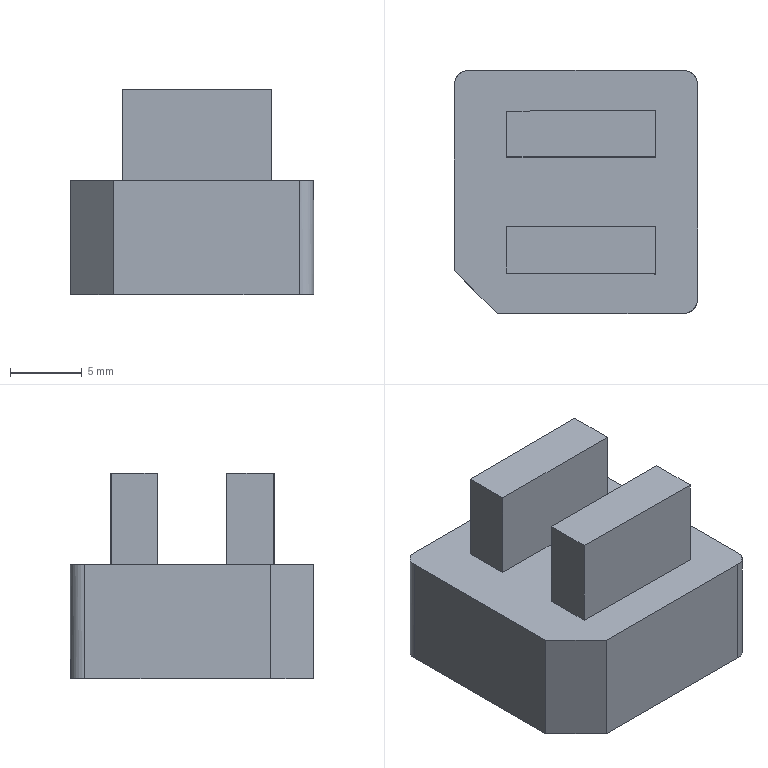NC program | PowerMill | posted with a generic post | part box 17 x 17 x 14.396 mm
Lines 2717 to 3695 of 69084:
N2814 M6
N2815 S18000 M03
N2816 G00 G90 X0.0 Y0.0
N2817 G43 Z9.7958 H15
N2818
N2819 G05 P10000 R4
N2820 X1.635 Y-8.1486
N2821 Z0.8391
N2822 G01 Z-0.3609 F3000.0
N2823 X1.6437 Y-8.1314 F5000.0
N2824 G03 X1.5675 Y-7.8985 I-0.1545 J0.0783
N2825 G01 X0.2111 Y-7.2114
N2826 X-4.8545 Y-7.1849
N2827 X-5.2767 Y-7.1304
N2828 X-5.6576 Y-6.9652
N2829 X-6.1064 Y-6.5431
N2830 X-6.3115 Y-6.1209
N2831 X-6.3761 Y-5.6988
N2832 X-6.3724 Y-2.3217
N2833 X-6.2796 Y-1.8996
N2834 X-6.1209 Y-1.592
N2835 X-6.0357 Y-1.4775
N2836 X-5.6988 Y-1.1748
N2837 X-5.4786 Y-1.0553
N2838 X-5.2767 Y-0.9836
N2839 X-4.8545 Y-0.9292
N2840 X5.2767
N2841 X5.6988 Y-0.9368
N2842 X6.1209 Y-1.0428
N2843 X6.5431 Y-1.3066
N2844 X6.7076 Y-1.4775
N2845 X6.9516 Y-1.8996
N2846 X7.0443 Y-2.3217
N2847 X7.0482 Y-5.6988
N2848 X6.9988 Y-6.1209
N2849 X6.8147 Y-6.5431
N2850 X6.5431 Y-6.8619
N2851 X6.4127 Y-6.9652
N2852 X6.1209 Y-7.1257
N2853 X5.6988 Y-7.2318
N2854 X5.2767 Y-7.238
N2855 X0.2111 Y-7.2114
N2856 G00 Z5.7953
N2857 G01 X-1.9723 Y-0.8992 F10000.0
N2858 G00 Z-0.1109
N2859 G01 X-2.2978 Z-0.1166 F3000.0
N2860 X-4.8545 Z-0.1612
N2861 X-4.8584 Y-0.8994
N2862 X-5.147 Y-0.9366 Z-0.1663
N2863 X-5.1478 Y-0.9292 Z-0.1665
N2864 X-5.093 Y-0.3731 Z-0.1762
N2865 X-4.9308 Y0.1615 Z-0.186
N2866 X-4.6675 Y0.6542 Z-0.1957
N2867 X-4.4661 Y0.8996 Z-0.2012
N2868 X-0.1294 Y0.8995 Z-0.2769
N2869 X0.0719 Y0.6542 Z-0.2825
N2870 X0.3353 Y0.1615 Z-0.2922
N2871 X0.4975 Y-0.3731 Z-0.302
N2872 X0.5493 Y-0.8992 Z-0.3112
N2873 X-2.2978 Z-0.3609
N2874 Y-0.9292
N2875 X-4.8756 Y0.9331 F5000.0
N2876 X-5.2767 Y0.9986
N2877 X-5.4279 Y1.0553
N2878 X-5.6988 Y1.2093
N2879 X-5.9855 Y1.4775
N2880 X-6.1209 Y1.6719
N2881 X-6.2295 Y1.8996
N2882 X-6.3223 Y2.3217
N2883 X-6.3249 Y5.6988
N2884 X-6.2454 Y6.1209
N2885 X-6.1209 Y6.3928
N2886 X-6.0204 Y6.5431
N2887 X-5.6988 Y6.8554
N2888 X-5.5201 Y6.9652
N2889 X-5.2767 Y7.0661
N2890 X-4.8545 Y7.135
N2891 X5.2767 Y7.1883
N2892 X5.6988 Y7.1821
N2893 X6.1209 Y7.0759
N2894 X6.3374 Y6.9652
N2895 X6.5431 Y6.8122
N2896 X6.7817 Y6.5431
N2897 X6.9652 Y6.1816
N2898 X7.0481 Y5.6988
N2899 X7.0442 Y2.3217
N2900 X6.9652 Y1.9374
N2901 X6.7074 Y1.4775
N2902 X6.5431 Y1.3068
N2903 X6.1499 Y1.0553
N2904 X5.6988 Y0.9369
N2905 X5.2767 Y0.9294
N2906 X-4.8545 Y0.9296
N2907 X-4.8756 Y0.9331
N2908 X-6.6768 Y-0.018 Z-0.5078
N2909 X-6.5047 Y-0.1041
N2910 X-4.8545 Y-0.9292
N2911 X5.2767
N2912 X5.6988 Y-0.9368
N2913 X6.1209 Y-1.0428
N2914 X6.5431 Y-1.3066
N2915 X6.7076 Y-1.4775
N2916 X6.9516 Y-1.8996
N2917 X7.0443 Y-2.3217
N2918 X7.0482 Y-5.6988
N2919 X6.9988 Y-6.1209
N2920 X6.8147 Y-6.5431
N2921 X6.5431 Y-6.8619
N2922 X6.4127 Y-6.9652
N2923 X6.1209 Y-7.1257
N2924 X5.6988 Y-7.2318
N2925 X5.2767 Y-7.238
N2926 X-4.8545 Y-7.1849
N2927 X-5.2767 Y-7.1304
N2928 X-5.6576 Y-6.9652
N2929 X-6.1064 Y-6.5431
N2930 X-6.3115 Y-6.1209
N2931 X-6.3761 Y-5.6988
N2932 X-6.3724 Y-2.3217
N2933 X-6.2796 Y-1.8996
N2934 X-6.1209 Y-1.592
N2935 X-6.0357 Y-1.4775
N2936 X-5.6988 Y-1.1748
N2937 X-5.4786 Y-1.0553
N2938 X-5.2767 Y-0.9836
N2939 X-4.8545 Y-0.9292
N2940 X-2.0017 Y-0.8992 Z-0.2578
N2941 X-2.3239 Z-0.2634 F3000.0
N2942 X-4.8545 Z-0.3075
N2943 X-4.8584 Y-0.8994 Z-0.3076
N2944 X-5.1729 Y-0.9399 Z-0.3131
N2945 X-5.1739 Y-0.9292 Z-0.3133
N2946 X-5.1192 Y-0.3731 Z-0.3231
N2947 X-4.957 Y0.1615 Z-0.3328
N2948 X-4.6936 Y0.6542 Z-0.3426
N2949 X-4.4922 Y0.8996 Z-0.3481
N2950 X-0.1556 Y0.8995 Z-0.4238
N2951 X0.0458 Y0.6542 Z-0.4293
N2952 X0.3091 Y0.1615 Z-0.4391
N2953 X0.4713 Y-0.3731 Z-0.4488
N2954 X0.5231 Y-0.8992 Z-0.4581
N2955 X-2.3239 Z-0.5078
N2956 Y-0.9292
N2957 X-4.9094 Y0.9386 F5000.0
N2958 X-5.2767 Y0.9986
N2959 X-5.4279 Y1.0553
N2960 X-5.6988 Y1.2093
N2961 X-5.9855 Y1.4775
N2962 X-6.1209 Y1.6719
N2963 X-6.2295 Y1.8996
N2964 X-6.3223 Y2.3217
N2965 X-6.3249 Y5.6988
N2966 X-6.2454 Y6.1209
N2967 X-6.1209 Y6.3928
N2968 X-6.0204 Y6.5431
N2969 X-5.6988 Y6.8554
N2970 X-5.5201 Y6.9652
N2971 X-5.2767 Y7.0661
N2972 X-4.8545 Y7.135
N2973 X5.2767 Y7.1883
N2974 X5.6988 Y7.1821
N2975 X6.1209 Y7.0759
N2976 X6.3374 Y6.9652
N2977 X6.5431 Y6.8122
N2978 X6.7817 Y6.5431
N2979 X6.9652 Y6.1816
N2980 X7.0481 Y5.6988
N2981 X7.0442 Y2.3217
N2982 X6.9652 Y1.9374
N2983 X6.7074 Y1.4775
N2984 X6.5431 Y1.3068
N2985 X6.1499 Y1.0553
N2986 X5.6988 Y0.9369
N2987 X5.2767 Y0.9294
N2988 X-4.8545 Y0.9296
N2989 X-4.9094 Y0.9386
N2990 X-6.6768 Y-0.018 Z-0.6546
N2991 X-6.5047 Y-0.1041
N2992 X-4.8545 Y-0.9291
N2993 X5.2767
N2994 X5.6988 Y-0.9368
N2995 X6.1209 Y-1.0428
N2996 X6.5431 Y-1.3066
N2997 X6.7076 Y-1.4775
N2998 X6.9516 Y-1.8996
N2999 X7.0443 Y-2.3217
N3000 X7.0482 Y-5.6988
N3001 X6.9988 Y-6.1209
N3002 X6.8147 Y-6.5431
N3003 X6.5431 Y-6.8619
N3004 X6.4127 Y-6.9652
N3005 X6.1209 Y-7.1257
N3006 X5.6988 Y-7.2318
N3007 X5.2767 Y-7.238
N3008 X-4.8545 Y-7.1849
N3009 X-5.2767 Y-7.1304
N3010 X-5.6576 Y-6.9652
N3011 X-6.1064 Y-6.5431
N3012 X-6.3115 Y-6.1209
N3013 X-6.3761 Y-5.6988
N3014 X-6.3724 Y-2.3217
N3015 X-6.2796 Y-1.8996
N3016 X-6.1209 Y-1.592
N3017 X-6.0357 Y-1.4775
N3018 X-5.6988 Y-1.1748
N3019 X-5.4786 Y-1.0553
N3020 X-5.2767 Y-0.9836
N3021 X-4.8545 Y-0.9291
N3022 X-2.0017 Y-0.8991 Z-0.4046
N3023 X-2.3239 Z-0.4103 F3000.0
N3024 X-4.8545 Z-0.4544
N3025 X-4.8584 Y-0.8994 Z-0.4545
N3026 X-5.1729 Y-0.9399 Z-0.46
N3027 X-5.1739 Y-0.9291 Z-0.4602
N3028 X-5.1192 Y-0.3731 Z-0.47
N3029 X-4.957 Y0.1615 Z-0.4797
N3030 X-4.6936 Y0.6542 Z-0.4895
N3031 X-4.4922 Y0.8996 Z-0.495
N3032 X-0.1556 Y0.8995 Z-0.5707
N3033 X0.0458 Y0.6542 Z-0.5762
N3034 X0.3091 Y0.1615 Z-0.586
N3035 X0.4713 Y-0.3731 Z-0.5957
N3036 X0.5231 Y-0.8991 Z-0.605
N3037 X-2.3239 Z-0.6546
N3038 Y-0.9291
N3039 X-4.9094 Y0.9386 F5000.0
N3040 X-5.2767 Y0.9986
N3041 X-5.4279 Y1.0553
N3042 X-5.6988 Y1.2092
N3043 X-5.9855 Y1.4775
N3044 X-6.1209 Y1.6719
N3045 X-6.2295 Y1.8996
N3046 X-6.3223 Y2.3217
N3047 X-6.3249 Y5.6988
N3048 X-6.2454 Y6.1209
N3049 X-6.1209 Y6.3928
N3050 X-6.0204 Y6.5431
N3051 X-5.6988 Y6.8554
N3052 X-5.5201 Y6.9652
N3053 X-5.2767 Y7.0661
N3054 X-4.8545 Y7.1351
N3055 X5.2767 Y7.1883
N3056 X5.6988 Y7.1821
N3057 X6.1209 Y7.0759
N3058 X6.3375 Y6.9652
N3059 X6.5431 Y6.8122
N3060 X6.7817 Y6.5431
N3061 X6.9652 Y6.1816
N3062 X7.0481 Y5.6988
N3063 X7.0442 Y2.3217
N3064 X6.9652 Y1.9374
N3065 X6.7074 Y1.4775
N3066 X6.5431 Y1.3068
N3067 X6.1499 Y1.0553
N3068 X5.6988 Y0.9369
N3069 X5.2767 Y0.9294
N3070 X-4.8545 Y0.9296
N3071 X-4.9094 Y0.9386
N3072 X-6.6768 Y-0.018 Z-0.8015
N3073 X-6.5047 Y-0.1041
N3074 X-4.8545 Y-0.9291
N3075 X5.2767
N3076 X5.6988 Y-0.9367
N3077 X6.1209 Y-1.0428
N3078 X6.5431 Y-1.3066
N3079 X6.7076 Y-1.4775
N3080 X6.9516 Y-1.8996
N3081 X7.0443 Y-2.3217
N3082 X7.0482 Y-5.6988
N3083 X6.9988 Y-6.1209
N3084 X6.8147 Y-6.5431
N3085 X6.5431 Y-6.8619
N3086 X6.4127 Y-6.9652
N3087 X6.1209 Y-7.1257
N3088 X5.6988 Y-7.2318
N3089 X5.2767 Y-7.238
N3090 X-4.8545 Y-7.1849
N3091 X-5.2767 Y-7.1304
N3092 X-5.6576 Y-6.9652
N3093 X-6.1064 Y-6.5431
N3094 X-6.3115 Y-6.1209
N3095 X-6.3761 Y-5.6988
N3096 X-6.3724 Y-2.3217
N3097 X-6.2797 Y-1.8996
N3098 X-6.1209 Y-1.592
N3099 X-6.0357 Y-1.4775
N3100 X-5.6988 Y-1.1748
N3101 X-5.4786 Y-1.0553
N3102 X-5.2767 Y-0.9836
N3103 X-4.8545 Y-0.9291
N3104 X-2.0017 Y-0.8991 Z-0.5515
N3105 X-2.3239 Z-0.5572 F3000.0
N3106 X-4.8545 Z-0.6013
N3107 X-4.8584 Y-0.8994 Z-0.6014
N3108 X-5.1729 Y-0.9399 Z-0.6069
N3109 X-5.1739 Y-0.9291 Z-0.6071
N3110 X-5.1192 Y-0.3731 Z-0.6169
N3111 X-4.957 Y0.1615 Z-0.6266
N3112 X-4.6936 Y0.6542 Z-0.6364
N3113 X-4.4922 Y0.8996 Z-0.6419
N3114 X-0.1556 Y0.8995 Z-0.7176
N3115 X0.0457 Y0.6542 Z-0.7231
N3116 X0.3091 Y0.1615 Z-0.7329
N3117 X0.4713 Y-0.3731 Z-0.7426
N3118 X0.5231 Y-0.8991 Z-0.7518
N3119 X-2.3239 Z-0.8015
N3120 Y-0.9291
N3121 X-4.9094 Y0.9386 F5000.0
N3122 X-5.2767 Y0.9986
N3123 X-5.4279 Y1.0553
N3124 X-5.6988 Y1.2092
N3125 X-5.9855 Y1.4775
N3126 X-6.1209 Y1.6719
N3127 X-6.2295 Y1.8996
N3128 X-6.3223 Y2.3217
N3129 X-6.3249 Y5.6988
N3130 X-6.2454 Y6.1209
N3131 X-6.1209 Y6.3928
N3132 X-6.0204 Y6.5431
N3133 X-5.6988 Y6.8554
N3134 X-5.5201 Y6.9652
N3135 X-5.2767 Y7.0661
N3136 X-4.8545 Y7.1351
N3137 X5.2767 Y7.1883
N3138 X5.6988 Y7.1821
N3139 X6.1209 Y7.0759
N3140 X6.3375 Y6.9652
N3141 X6.5431 Y6.8122
N3142 X6.7817 Y6.5431
N3143 X6.9652 Y6.1816
N3144 X7.0481 Y5.6988
N3145 X7.0442 Y2.3217
N3146 X6.9652 Y1.9374
N3147 X6.7074 Y1.4775
N3148 X6.5431 Y1.3068
N3149 X6.1499 Y1.0553
N3150 X5.6988 Y0.9369
N3151 X5.2767 Y0.9294
N3152 X-4.8545 Y0.9296
N3153 X-4.9094 Y0.9386
N3154 X-6.6768 Y-0.018 Z-0.9484
N3155 X-6.5047 Y-0.1041
N3156 X-4.8545 Y-0.9291
N3157 X5.2767
N3158 X5.6988 Y-0.9367
N3159 X6.1209 Y-1.0428
N3160 X6.5431 Y-1.3066
N3161 X6.7076 Y-1.4775
N3162 X6.9516 Y-1.8996
N3163 X7.0443 Y-2.3217
N3164 X7.0482 Y-5.6988
N3165 X6.9988 Y-6.1209
N3166 X6.8147 Y-6.5431
N3167 X6.5431 Y-6.8619
N3168 X6.4127 Y-6.9652
N3169 X6.1209 Y-7.1257
N3170 X5.6988 Y-7.2318
N3171 X5.2767 Y-7.238
N3172 X-4.8545 Y-7.1849
N3173 X-5.2767 Y-7.1304
N3174 X-5.6576 Y-6.9652
N3175 X-6.1064 Y-6.5431
N3176 X-6.3115 Y-6.1209
N3177 X-6.3761 Y-5.6988
N3178 X-6.3724 Y-2.3217
N3179 X-6.2797 Y-1.8996
N3180 X-6.1209 Y-1.592
N3181 X-6.0357 Y-1.4775
N3182 X-5.6988 Y-1.1748
N3183 X-5.4786 Y-1.0553
N3184 X-5.2767 Y-0.9836
N3185 X-4.8545 Y-0.9291
N3186 X-2.0017 Y-0.8991 Z-0.6984
N3187 X-2.3239 Z-0.704 F3000.0
N3188 X-4.8545 Z-0.7482
N3189 X-4.8584 Y-0.8994 Z-0.7483
N3190 X-5.1729 Y-0.9399 Z-0.7538
N3191 X-5.1739 Y-0.9291 Z-0.754
N3192 X-5.1192 Y-0.3731 Z-0.7637
N3193 X-4.957 Y0.1615 Z-0.7735
N3194 X-4.6936 Y0.6542 Z-0.7832
N3195 X-4.4923 Y0.8996 Z-0.7888
N3196 X-0.1556 Y0.8995 Z-0.8645
N3197 X0.0457 Y0.6542 Z-0.87
N3198 X0.3091 Y0.1615 Z-0.8797
N3199 X0.4713 Y-0.3731 Z-0.8895
N3200 X0.5231 Y-0.8991 Z-0.8987
N3201 X-2.3239 Z-0.9484
N3202 Y-0.9291
N3203 X-4.9094 Y0.9386 F5000.0
N3204 X-5.2767 Y0.9986
N3205 X-5.4279 Y1.0553
N3206 X-5.6988 Y1.2092
N3207 X-5.9855 Y1.4775
N3208 X-6.1209 Y1.6719
N3209 X-6.2295 Y1.8996
N3210 X-6.3223 Y2.3217
N3211 X-6.3249 Y5.6988
N3212 X-6.2454 Y6.1209
N3213 X-6.1209 Y6.3928
N3214 X-6.0204 Y6.5431
N3215 X-5.6988 Y6.8554
N3216 X-5.5202 Y6.9652
N3217 X-5.2767 Y7.0661
N3218 X-4.8545 Y7.1351
N3219 X5.2767 Y7.1883
N3220 X5.6988 Y7.1821
N3221 X6.1209 Y7.0759
N3222 X6.3375 Y6.9652
N3223 X6.5431 Y6.8122
N3224 X6.7817 Y6.5431
N3225 X6.9652 Y6.1816
N3226 X7.0481 Y5.6988
N3227 X7.0442 Y2.3217
N3228 X6.9652 Y1.9374
N3229 X6.7074 Y1.4775
N3230 X6.5431 Y1.3068
N3231 X6.1499 Y1.0553
N3232 X5.6988 Y0.9369
N3233 X5.2767 Y0.9294
N3234 X-4.8545 Y0.9296
N3235 X-4.9094 Y0.9386
N3236 X-6.6768 Y-0.018 Z-1.0953
N3237 X-6.5047 Y-0.1041
N3238 X-4.8545 Y-0.9291
N3239 X5.2767
N3240 X5.6988 Y-0.9367
N3241 X6.1209 Y-1.0428
N3242 X6.5431 Y-1.3065
N3243 X6.7076 Y-1.4775
N3244 X6.9516 Y-1.8996
N3245 X7.0443 Y-2.3217
N3246 X7.0482 Y-5.6988
N3247 X6.9988 Y-6.1209
N3248 X6.8147 Y-6.5431
N3249 X6.5431 Y-6.8619
N3250 X6.4127 Y-6.9652
N3251 X6.1209 Y-7.1257
N3252 X5.6988 Y-7.2318
N3253 X5.2767 Y-7.238
N3254 X-4.8545 Y-7.1849
N3255 X-5.2767 Y-7.1304
N3256 X-5.6576 Y-6.9652
N3257 X-6.1064 Y-6.5431
N3258 X-6.3115 Y-6.1209
N3259 X-6.3761 Y-5.6988
N3260 X-6.3724 Y-2.3217
N3261 X-6.2797 Y-1.8996
N3262 X-6.1209 Y-1.592
N3263 X-6.0357 Y-1.4775
N3264 X-5.6988 Y-1.1748
N3265 X-5.4786 Y-1.0553
N3266 X-5.2767 Y-0.9836
N3267 X-4.8545 Y-0.9291
N3268 X-2.0017 Y-0.8991 Z-0.8453
N3269 X-2.324 Z-0.8509 F3000.0
N3270 X-4.8545 Z-0.8951
N3271 X-4.8584 Y-0.8994 Z-0.8952
N3272 X-5.1729 Y-0.9399 Z-0.9007
N3273 X-5.174 Y-0.9291 Z-0.9009
N3274 X-5.1192 Y-0.3731 Z-0.9106
N3275 X-4.957 Y0.1615 Z-0.9204
N3276 X-4.6936 Y0.6542 Z-0.9301
N3277 X-4.4923 Y0.8996 Z-0.9357
N3278 X-0.1556 Y0.8995 Z-1.0114
N3279 X0.0457 Y0.6542 Z-1.0169
N3280 X0.3091 Y0.1615 Z-1.0266
N3281 X0.4713 Y-0.3731 Z-1.0364
N3282 X0.5231 Y-0.8991 Z-1.0456
N3283 X-2.324 Z-1.0953
N3284 Y-0.9291
N3285 X-4.9094 Y0.9386 F5000.0
N3286 X-5.2767 Y0.9986
N3287 X-5.4279 Y1.0553
N3288 X-5.6988 Y1.2092
N3289 X-5.9855 Y1.4775
N3290 X-6.1209 Y1.6718
N3291 X-6.2295 Y1.8996
N3292 X-6.3223 Y2.3217
N3293 X-6.3249 Y5.6988
N3294 X-6.2454 Y6.1209
N3295 X-6.1209 Y6.3928
N3296 X-6.0204 Y6.5431
N3297 X-5.6988 Y6.8554
N3298 X-5.5202 Y6.9652
N3299 X-5.2767 Y7.0661
N3300 X-4.8545 Y7.1351
N3301 X5.2767 Y7.1883
N3302 X5.6988 Y7.1821
N3303 X6.1209 Y7.0759
N3304 X6.3375 Y6.9652
N3305 X6.5431 Y6.8122
N3306 X6.7817 Y6.5431
N3307 X6.9652 Y6.1816
N3308 X7.0481 Y5.6988
N3309 X7.0442 Y2.3217
N3310 X6.9652 Y1.9374
N3311 X6.7074 Y1.4775
N3312 X6.5431 Y1.3068
N3313 X6.1499 Y1.0553
N3314 X5.6988 Y0.9369
N3315 X5.2767 Y0.9294
N3316 X-4.8545 Y0.9296
N3317 X-4.9094 Y0.9386
N3318 X-6.6768 Y-0.018 Z-1.2422
N3319 X-6.5047 Y-0.1041
N3320 X-4.8545 Y-0.9291
N3321 X5.2767
N3322 X5.6988 Y-0.9367
N3323 X6.1209 Y-1.0428
N3324 X6.5431 Y-1.3065
N3325 X6.7076 Y-1.4775
N3326 X6.9516 Y-1.8996
N3327 X7.0443 Y-2.3217
N3328 X7.0482 Y-5.6988
N3329 X6.9988 Y-6.1209
N3330 X6.8147 Y-6.5431
N3331 X6.5431 Y-6.8619
N3332 X6.4127 Y-6.9652
N3333 X6.1209 Y-7.1257
N3334 X5.6988 Y-7.2318
N3335 X5.2767 Y-7.238
N3336 X-4.8545 Y-7.1849
N3337 X-5.2767 Y-7.1304
N3338 X-5.6576 Y-6.9652
N3339 X-6.1064 Y-6.5431
N3340 X-6.3115 Y-6.1209
N3341 X-6.3761 Y-5.6988
N3342 X-6.3724 Y-2.3217
N3343 X-6.2797 Y-1.8996
N3344 X-6.1209 Y-1.592
N3345 X-6.0357 Y-1.4775
N3346 X-5.6988 Y-1.1748
N3347 X-5.4786 Y-1.0553
N3348 X-5.2767 Y-0.9836
N3349 X-4.8545 Y-0.9291
N3350 X-2.0017 Y-0.8991 Z-0.9922
N3351 X-2.324 Z-0.9978 F3000.0
N3352 X-4.8545 Z-1.042
N3353 X-4.8584 Y-0.8994
N3354 X-5.1729 Y-0.9399 Z-1.0476
N3355 X-5.174 Y-0.9291 Z-1.0478
N3356 X-5.1192 Y-0.3731 Z-1.0575
N3357 X-4.957 Y0.1615 Z-1.0673
N3358 X-4.6936 Y0.6542 Z-1.077
N3359 X-4.4923 Y0.8996 Z-1.0825
N3360 X-0.1556 Y0.8995 Z-1.1582
N3361 X0.0457 Y0.6542 Z-1.1638
N3362 X0.3091 Y0.1615 Z-1.1735
N3363 X0.4713 Y-0.3731 Z-1.1833
N3364 X0.5231 Y-0.8991 Z-1.1925
N3365 X-2.324 Z-1.2422
N3366 Y-0.9291
N3367 X-4.9094 Y0.9386 F5000.0
N3368 X-5.2767 Y0.9986
N3369 X-5.4279 Y1.0553
N3370 X-5.6988 Y1.2092
N3371 X-5.9855 Y1.4775
N3372 X-6.1209 Y1.6718
N3373 X-6.2295 Y1.8996
N3374 X-6.3224 Y2.3217
N3375 X-6.3249 Y5.6988
N3376 X-6.2454 Y6.1209
N3377 X-6.1209 Y6.3928
N3378 X-6.0204 Y6.5431
N3379 X-5.6988 Y6.8554
N3380 X-5.5202 Y6.9652
N3381 X-5.2767 Y7.0661
N3382 X-4.8545 Y7.1351
N3383 X5.2767 Y7.1883
N3384 X5.6988 Y7.1821
N3385 X6.1209 Y7.0759
N3386 X6.3375 Y6.9652
N3387 X6.5431 Y6.8122
N3388 X6.7817 Y6.5431
N3389 X6.9652 Y6.1816
N3390 X7.0481 Y5.6988
N3391 X7.0442 Y2.3217
N3392 X6.9652 Y1.9374
N3393 X6.7075 Y1.4775
N3394 X6.5431 Y1.3068
N3395 X6.1499 Y1.0553
N3396 X5.6988 Y0.9369
N3397 X5.2767 Y0.9294
N3398 X-4.8545 Y0.9296
N3399 X-4.9094 Y0.9386
N3400 X-6.6768 Y-0.018 Z-1.3891
N3401 X-6.5047 Y-0.1041
N3402 X-4.8545 Y-0.9291
N3403 X5.2767
N3404 X5.6988 Y-0.9367
N3405 X6.1209 Y-1.0428
N3406 X6.5431 Y-1.3065
N3407 X6.7076 Y-1.4775
N3408 X6.9516 Y-1.8996
N3409 X7.0443 Y-2.3217
N3410 X7.0482 Y-5.6988
N3411 X6.9988 Y-6.1209
N3412 X6.8147 Y-6.5431
N3413 X6.5431 Y-6.8619
N3414 X6.4127 Y-6.9652
N3415 X6.1209 Y-7.1257
N3416 X5.6988 Y-7.2318
N3417 X5.2767 Y-7.238
N3418 X-4.8545 Y-7.1849
N3419 X-5.2767 Y-7.1304
N3420 X-5.6576 Y-6.9652
N3421 X-6.1064 Y-6.5431
N3422 X-6.3115 Y-6.1209
N3423 X-6.3761 Y-5.6988
N3424 X-6.3724 Y-2.3217
N3425 X-6.2797 Y-1.8996
N3426 X-6.1209 Y-1.592
N3427 X-6.0357 Y-1.4775
N3428 X-5.6988 Y-1.1748
N3429 X-5.4786 Y-1.0553
N3430 X-5.2767 Y-0.9836
N3431 X-4.8545 Y-0.9291
N3432 X-2.0017 Y-0.8991 Z-1.1391
N3433 X-2.324 Z-1.1447 F3000.0
N3434 X-4.8545 Z-1.1888
N3435 X-4.8584 Y-0.8994 Z-1.1889
N3436 X-5.1729 Y-0.9399 Z-1.1944
N3437 X-5.174 Y-0.9291 Z-1.1946
N3438 X-5.1192 Y-0.3731 Z-1.2044
N3439 X-4.957 Y0.1615 Z-1.2141
N3440 X-4.6937 Y0.6542 Z-1.2239
N3441 X-4.4923 Y0.8996 Z-1.2294
N3442 X-0.1556 Y0.8995 Z-1.3051
N3443 X0.0457 Y0.6542 Z-1.3106
N3444 X0.3091 Y0.1615 Z-1.3204
N3445 X0.4713 Y-0.3731 Z-1.3301
N3446 X0.5231 Y-0.8991 Z-1.3394
N3447 X-2.324 Z-1.3891
N3448 Y-0.9291
N3449 X-4.9094 Y0.9386 F5000.0
N3450 X-5.2767 Y0.9986
N3451 X-5.4279 Y1.0553
N3452 X-5.6988 Y1.2092
N3453 X-5.9855 Y1.4775
N3454 X-6.1209 Y1.6718
N3455 X-6.2296 Y1.8996
N3456 X-6.3224 Y2.3217
N3457 X-6.3249 Y5.6988
N3458 X-6.2454 Y6.1209
N3459 X-6.1209 Y6.3928
N3460 X-6.0204 Y6.5431
N3461 X-5.6988 Y6.8554
N3462 X-5.5202 Y6.9652
N3463 X-5.2767 Y7.0661
N3464 X-4.8545 Y7.1351
N3465 X5.2767 Y7.1883
N3466 X5.6988 Y7.1821
N3467 X6.1209 Y7.0759
N3468 X6.3375 Y6.9652
N3469 X6.5431 Y6.8122
N3470 X6.7817 Y6.5431
N3471 X6.9652 Y6.1816
N3472 X7.0481 Y5.6988
N3473 X7.0442 Y2.3217
N3474 X6.9652 Y1.9374
N3475 X6.7075 Y1.4775
N3476 X6.5431 Y1.3068
N3477 X6.1499 Y1.0553
N3478 X5.6988 Y0.9369
N3479 X5.2767 Y0.9294
N3480 X-4.8545 Y0.9296
N3481 X-4.9094 Y0.9386
N3482 X-6.6768 Y-0.018 Z-1.5359
N3483 X-6.5047 Y-0.1041
N3484 X-4.8545 Y-0.9291
N3485 X5.2767
N3486 X5.6988 Y-0.9367
N3487 X6.1209 Y-1.0428
N3488 X6.5431 Y-1.3065
N3489 X6.7076 Y-1.4775
N3490 X6.9516 Y-1.8996
N3491 X7.0443 Y-2.3217
N3492 X7.0482 Y-5.6988
N3493 X6.9988 Y-6.1209
N3494 X6.8147 Y-6.5431
N3495 X6.5431 Y-6.8619
N3496 X6.4127 Y-6.9652
N3497 X6.1209 Y-7.1257
N3498 X5.6988 Y-7.2318
N3499 X5.2767 Y-7.238
N3500 X-4.8545 Y-7.1849
N3501 X-5.2767 Y-7.1304
N3502 X-5.6576 Y-6.9652
N3503 X-6.1064 Y-6.5431
N3504 X-6.3115 Y-6.1209
N3505 X-6.3761 Y-5.6988
N3506 X-6.3724 Y-2.3217
N3507 X-6.2797 Y-1.8996
N3508 X-6.1209 Y-1.592
N3509 X-6.0357 Y-1.4775
N3510 X-5.6988 Y-1.1748
N3511 X-5.4786 Y-1.0553
N3512 X-5.2767 Y-0.9836
N3513 X-4.8545 Y-0.9291
N3514 X-2.0017 Y-0.8991 Z-1.2859
N3515 X-2.324 Z-1.2916 F3000.0
N3516 X-4.8545 Z-1.3357
N3517 X-4.8584 Y-0.8994 Z-1.3358
N3518 X-5.1729 Y-0.9399 Z-1.3413
N3519 X-5.174 Y-0.9291 Z-1.3415
N3520 X-5.1192 Y-0.3731 Z-1.3513
N3521 X-4.957 Y0.1615 Z-1.361
N3522 X-4.6937 Y0.6542 Z-1.3708
N3523 X-4.4923 Y0.8996 Z-1.3763
N3524 X-0.1556 Y0.8995 Z-1.452
N3525 X0.0457 Y0.6542 Z-1.4575
N3526 X0.3091 Y0.1615 Z-1.4673
N3527 X0.4713 Y-0.3731 Z-1.477
N3528 X0.5231 Y-0.8991 Z-1.4863
N3529 X-2.324 Z-1.5359
N3530 Y-0.9291
N3531 X-4.9094 Y0.9386 F5000.0
N3532 X-5.2767 Y0.9986
N3533 X-5.4279 Y1.0553
N3534 X-5.6988 Y1.2092
N3535 X-5.9855 Y1.4775
N3536 X-6.1209 Y1.6718
N3537 X-6.2296 Y1.8996
N3538 X-6.3224 Y2.3217
N3539 X-6.3249 Y5.6988
N3540 X-6.2454 Y6.1209
N3541 X-6.1209 Y6.3928
N3542 X-6.0204 Y6.5431
N3543 X-5.6988 Y6.8554
N3544 X-5.5202 Y6.9652
N3545 X-5.2767 Y7.0661
N3546 X-4.8545 Y7.1351
N3547 X5.2767 Y7.1883
N3548 X5.6988 Y7.1821
N3549 X6.1209 Y7.0759
N3550 X6.3375 Y6.9652
N3551 X6.5431 Y6.8122
N3552 X6.7817 Y6.5431
N3553 X6.9652 Y6.1816
N3554 X7.0481 Y5.6988
N3555 X7.0442 Y2.3217
N3556 X6.9652 Y1.9374
N3557 X6.7075 Y1.4775
N3558 X6.5431 Y1.3068
N3559 X6.1499 Y1.0553
N3560 X5.6988 Y0.9369
N3561 X5.2767 Y0.9294
N3562 X-4.8545 Y0.9296
N3563 X-4.9094 Y0.9386
N3564 X-6.6768 Y-0.018 Z-1.6828
N3565 X-6.5047 Y-0.1041
N3566 X-4.8545 Y-0.9291
N3567 X5.2767
N3568 X5.6988 Y-0.9367
N3569 X6.1209 Y-1.0428
N3570 X6.5431 Y-1.3065
N3571 X6.7076 Y-1.4775
N3572 X6.9516 Y-1.8996
N3573 X7.0443 Y-2.3217
N3574 X7.0482 Y-5.6988
N3575 X6.9988 Y-6.1209
N3576 X6.8147 Y-6.5431
N3577 X6.5431 Y-6.8619
N3578 X6.4127 Y-6.9652
N3579 X6.1209 Y-7.1257
N3580 X5.6988 Y-7.2318
N3581 X5.2767 Y-7.238
N3582 X-4.8545 Y-7.1849
N3583 X-5.2767 Y-7.1304
N3584 X-5.6576 Y-6.9652
N3585 X-6.1064 Y-6.5431
N3586 X-6.3115 Y-6.1209
N3587 X-6.3761 Y-5.6988
N3588 X-6.3724 Y-2.3217
N3589 X-6.2797 Y-1.8996
N3590 X-6.1209 Y-1.592
N3591 X-6.0357 Y-1.4775
N3592 X-5.6988 Y-1.1748
N3593 X-5.4786 Y-1.0553
N3594 X-5.2767 Y-0.9836
N3595 X-4.8545 Y-0.9291
N3596 X-2.0017 Y-0.8991 Z-1.4328
N3597 X-2.324 Z-1.4385 F3000.0
N3598 X-4.8545 Z-1.4826
N3599 X-4.8584 Y-0.8994 Z-1.4827
N3600 X-5.1729 Y-0.9399 Z-1.4882
N3601 X-5.174 Y-0.9291 Z-1.4884
N3602 X-5.1192 Y-0.3731 Z-1.4982
N3603 X-4.957 Y0.1615 Z-1.5079
N3604 X-4.6937 Y0.6542 Z-1.5177
N3605 X-4.4923 Y0.8996 Z-1.5232
N3606 X-0.1556 Y0.8995 Z-1.5989
N3607 X0.0457 Y0.6542 Z-1.6044
N3608 X0.3091 Y0.1615 Z-1.6142
N3609 X0.4713 Y-0.3731 Z-1.6239
N3610 X0.5231 Y-0.8991 Z-1.6331
N3611 X-2.324 Z-1.6828
N3612 Y-0.9291
N3613 X-4.9094 Y0.9386 F5000.0
N3614 X-5.2767 Y0.9986
N3615 X-5.4279 Y1.0553
N3616 X-5.6988 Y1.2092
N3617 X-5.9855 Y1.4775
N3618 X-6.1209 Y1.6718
N3619 X-6.2296 Y1.8996
N3620 X-6.3224 Y2.3217
N3621 X-6.3249 Y5.6988
N3622 X-6.2454 Y6.1209
N3623 X-6.1209 Y6.3928
N3624 X-6.0204 Y6.5431
N3625 X-5.6988 Y6.8554
N3626 X-5.5202 Y6.9652
N3627 X-5.2767 Y7.0661
N3628 X-4.8545 Y7.1351
N3629 X5.2767 Y7.1883
N3630 X5.6988 Y7.1821
N3631 X6.1209 Y7.0759
N3632 X6.3375 Y6.9652
N3633 X6.5431 Y6.8122
N3634 X6.7817 Y6.5431
N3635 X6.9652 Y6.1816
N3636 X7.0481 Y5.6988
N3637 X7.0442 Y2.3217
N3638 X6.9652 Y1.9374
N3639 X6.7075 Y1.4775
N3640 X6.5431 Y1.3068
N3641 X6.1499 Y1.0553
N3642 X5.6988 Y0.9369
N3643 X5.2767 Y0.9294
N3644 X-4.8545 Y0.9296
N3645 X-4.9094 Y0.9386
N3646 X-6.6768 Y-0.018 Z-1.8297
N3647 X-6.5047 Y-0.1041
N3648 X-4.8545 Y-0.9291
N3649 X5.2767
N3650 X5.6988 Y-0.9367
N3651 X6.1209 Y-1.0428
N3652 X6.5431 Y-1.3065
N3653 X6.7076 Y-1.4775
N3654 X6.9516 Y-1.8996
N3655 X7.0443 Y-2.3217
N3656 X7.0482 Y-5.6988
N3657 X6.9988 Y-6.1209
N3658 X6.8147 Y-6.5431
N3659 X6.5431 Y-6.8619
N3660 X6.4127 Y-6.9652
N3661 X6.1209 Y-7.1257
N3662 X5.6988 Y-7.2318
N3663 X5.2767 Y-7.238
N3664 X-4.8545 Y-7.1849
N3665 X-5.2767 Y-7.1304
N3666 X-5.6576 Y-6.9652
N3667 X-6.1064 Y-6.5431
N3668 X-6.3115 Y-6.1209
N3669 X-6.3761 Y-5.6988
N3670 X-6.3724 Y-2.3217
N3671 X-6.2797 Y-1.8996
N3672 X-6.1209 Y-1.592
N3673 X-6.0357 Y-1.4775
N3674 X-5.6988 Y-1.1748
N3675 X-5.4786 Y-1.0553
N3676 X-5.2767 Y-0.9836
N3677 X-4.8545 Y-0.9291
N3678 X-2.0017 Y-0.8991 Z-1.5797
N3679 X-2.324 Z-1.5853 F3000.0
N3680 X-4.8545 Z-1.6295
N3681 X-4.8584 Y-0.8994 Z-1.6296
N3682 X-5.1729 Y-0.9399 Z-1.6351
N3683 X-5.174 Y-0.9291 Z-1.6353
N3684 X-5.1192 Y-0.3731 Z-1.645
N3685 X-4.957 Y0.1615 Z-1.6548
N3686 X-4.6937 Y0.6542 Z-1.6645
N3687 X-4.4923 Y0.8996 Z-1.6701
N3688 X-0.1556 Y0.8995 Z-1.7458
N3689 X0.0457 Y0.6542 Z-1.7513
N3690 X0.3091 Y0.1615 Z-1.7611
N3691 X0.4713 Y-0.3731 Z-1.7708
N3692 X0.5231 Y-0.8991 Z-1.78
N3693 X-2.324 Z-1.8297
N3694 Y-0.9291
N3695 X-4.9094 Y0.9386 F5000.0
N3696 X-5.2767 Y0.9986
N3697 X-5.4279 Y1.0553
N3698 X-5.6988 Y1.2092
N3699 X-5.9855 Y1.4775
N3700 X-6.1209 Y1.6718
N3701 X-6.2296 Y1.8996
N3702 X-6.3224 Y2.3217
N3703 X-6.3249 Y5.6988
N3704 X-6.2454 Y6.1209
N3705 X-6.1209 Y6.3928
N3706 X-6.0204 Y6.5431
N3707 X-5.6988 Y6.8554
N3708 X-5.5202 Y6.9652
N3709 X-5.2767 Y7.0661
N3710 X-4.8545 Y7.1351
N3711 X5.2767 Y7.1883
N3712 X5.6988 Y7.1821
N3713 X6.1209 Y7.076
N3714 X6.3375 Y6.9652
N3715 X6.5431 Y6.8122
N3716 X6.7817 Y6.5431
N3717 X6.9652 Y6.1816
N3718 X7.0481 Y5.6988
N3719 X7.0442 Y2.3217
N3720 X6.9652 Y1.9374
N3721 X6.7075 Y1.4775
N3722 X6.5431 Y1.3068
N3723 X6.1499 Y1.0553
N3724 X5.6988 Y0.9369
N3725 X5.2767 Y0.9294
N3726 X-4.8545 Y0.9296
N3727 X-4.9094 Y0.9386
N3728 X-6.6768 Y-0.018 Z-1.9766
N3729 X-6.5047 Y-0.1041
N3730 X-4.8545 Y-0.9291
N3731 X5.2767
N3732 X5.6988 Y-0.9367
N3733 X6.1209 Y-1.0428
N3734 X6.5431 Y-1.3065
N3735 X6.7077 Y-1.4775
N3736 X6.9516 Y-1.8996
N3737 X7.0443 Y-2.3217
N3738 X7.0482 Y-5.6988
N3739 X6.9988 Y-6.1209
N3740 X6.8147 Y-6.5431
N3741 X6.5431 Y-6.8619
N3742 X6.4127 Y-6.9652
N3743 X6.1209 Y-7.1257
N3744 X5.6988 Y-7.2318
N3745 X5.2767 Y-7.238
N3746 X-4.8545 Y-7.1849
N3747 X-5.2767 Y-7.1304
N3748 X-5.6576 Y-6.9652
N3749 X-6.1064 Y-6.5431
N3750 X-6.3115 Y-6.1209
N3751 X-6.3761 Y-5.6988
N3752 X-6.3724 Y-2.3217
N3753 X-6.2797 Y-1.8996
N3754 X-6.1209 Y-1.592
N3755 X-6.0357 Y-1.4775
N3756 X-5.6988 Y-1.1748
N3757 X-5.4786 Y-1.0553
N3758 X-5.2767 Y-0.9836
N3759 X-4.8545 Y-0.9291
N3760 X-2.0017 Y-0.8991 Z-1.7266
N3761 X-2.324 Z-1.7322 F3000.0
N3762 X-4.8545 Z-1.7764
N3763 X-4.8584 Y-0.8994 Z-1.7765
N3764 X-5.1729 Y-0.9399 Z-1.782
N3765 X-5.174 Y-0.9291 Z-1.7822
N3766 X-5.1192 Y-0.3731 Z-1.7919
N3767 X-4.957 Y0.1615 Z-1.8017
N3768 X-4.6937 Y0.6542 Z-1.8114
N3769 X-4.4923 Y0.8996 Z-1.817
N3770 X-0.1556 Y0.8995 Z-1.8927
N3771 X0.0457 Y0.6542 Z-1.8982
N3772 X0.3091 Y0.1615 Z-1.9079
N3773 X0.4713 Y-0.3731 Z-1.9177
N3774 X0.5231 Y-0.8991 Z-1.9269
N3775 X-2.324 Z-1.9766
N3776 Y-0.9291
N3777 X-4.9094 Y0.9386 F5000.0
N3778 X-5.2767 Y0.9986
N3779 X-5.4279 Y1.0553
N3780 X-5.6988 Y1.2092
N3781 X-5.9855 Y1.4775
N3782 X-6.1209 Y1.6718
N3783 X-6.2296 Y1.8996
N3784 X-6.3224 Y2.3217
N3785 X-6.3249 Y5.6988
N3786 X-6.2454 Y6.1209
N3787 X-6.1209 Y6.3928
N3788 X-6.0204 Y6.5431
N3789 X-5.6988 Y6.8554
N3790 X-5.5202 Y6.9652
N3791 X-5.2767 Y7.0661
N3792 X-4.8545 Y7.1351